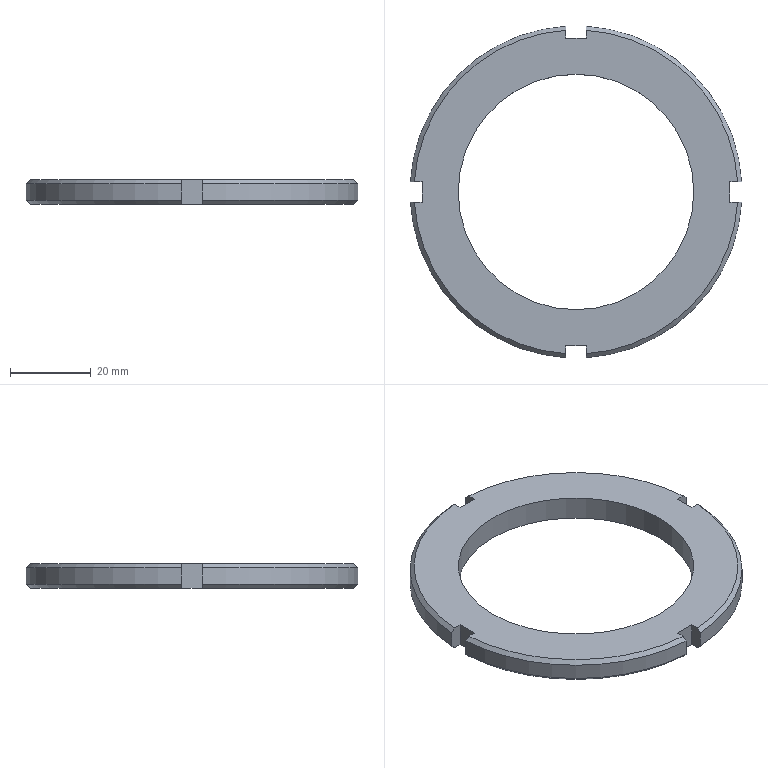Part | NX | features DATUM_CSYS 2, CHAMFER 1, EXTRUDE 1, HOLE PACKAGE 1, Pattern Face Feature 1, SIMPLE HOLE 1, SKETCH 1, SYMBOLIC_THREAD 1 | 1 solid | 27 faces | box 81.847 x 81.847 x 6 mm | volume 15157 mm3 | plane 14 | cone 8 | cylinder 5 | commonest cylinder face diameters 82 x4 58.154 x1
STEP:
#1=CARTESIAN_POINT('',(-2.5,40.924,5.));
#2=VERTEX_POINT('',#1);
#3=CARTESIAN_POINT('',(-2.5,40.924,1.));
#4=VERTEX_POINT('',#3);
#5=CARTESIAN_POINT('',(-2.5,40.924,6.));
#6=DIRECTION('',(0.,0.,-1.));
#7=VECTOR('',#6,1000.);
#8=LINE('',#5,#7);
#9=EDGE_CURVE('',#2,#4,#8,.T.);
#10=ORIENTED_EDGE('',*,*,#9,.T.);
#11=CARTESIAN_POINT('',(-40.924,2.5,1.));
#12=VERTEX_POINT('',#11);
#13=CARTESIAN_POINT('',(0.,0.,1.));
#14=DIRECTION('',(0.,0.,1.));
#15=DIRECTION('',(1.,0.,0.));
#16=AXIS2_PLACEMENT_3D('',#13,#14,#15);
#17=CIRCLE('',#16,41.);
#18=EDGE_CURVE('',#4,#12,#17,.T.);
#19=ORIENTED_EDGE('',*,*,#18,.T.);
#20=CARTESIAN_POINT('',(-40.924,2.5,5.));
#21=VERTEX_POINT('',#20);
#22=CARTESIAN_POINT('',(-40.924,2.5,6.));
#23=DIRECTION('',(0.,0.,-1.));
#24=VECTOR('',#23,1000.);
#25=LINE('',#22,#24);
#26=EDGE_CURVE('',#21,#12,#25,.T.);
#27=ORIENTED_EDGE('',*,*,#26,.F.);
#28=CARTESIAN_POINT('',(0.,0.,5.));
#29=DIRECTION('',(0.,0.,1.));
#30=DIRECTION('',(1.,0.,0.));
#31=AXIS2_PLACEMENT_3D('',#28,#29,#30);
#32=CIRCLE('',#31,41.);
#33=EDGE_CURVE('',#21,#2,#32,.F.);
#34=ORIENTED_EDGE('',*,*,#33,.T.);
#35=EDGE_LOOP('',(#10,#19,#27,#34));
#36=FACE_BOUND('',#35,.T.);
#37=CARTESIAN_POINT('',(0.,0.,6.));
#38=DIRECTION('',(0.,0.,-1.));
#39=DIRECTION('',(-1.,0.,0.));
#40=AXIS2_PLACEMENT_3D('',#37,#38,#39);
#41=CYLINDRICAL_SURFACE('',#40,41.);
#42=ADVANCED_FACE('',(#36),#41,.T.);
#43=CARTESIAN_POINT('',(2.5,40.924,5.));
#44=VERTEX_POINT('',#43);
#45=CARTESIAN_POINT('',(2.5,40.924,1.));
#46=VERTEX_POINT('',#45);
#47=CARTESIAN_POINT('',(2.5,40.924,6.));
#48=DIRECTION('',(0.,0.,-1.));
#49=VECTOR('',#48,1000.);
#50=LINE('',#47,#49);
#51=EDGE_CURVE('',#44,#46,#50,.T.);
#52=ORIENTED_EDGE('',*,*,#51,.T.);
#53=CARTESIAN_POINT('',(2.5,39.922,0.));
#54=VERTEX_POINT('',#53);
#55=CARTESIAN_POINT('',(2.5,40.924,1.));
#56=CARTESIAN_POINT('',(2.5,40.59,0.6667));
#57=CARTESIAN_POINT('',(2.5,40.256,0.3333));
#58=CARTESIAN_POINT('',(2.5,39.922,0.));
#59=B_SPLINE_CURVE_WITH_KNOTS('',3,(#55,#56,#57,#58),.UNSPECIFIED.,.F.,.F.,(4,4),(0.,0.001416),.UNSPECIFIED.);
#60=EDGE_CURVE('',#46,#54,#59,.T.);
#61=ORIENTED_EDGE('',*,*,#60,.T.);
#62=CARTESIAN_POINT('',(2.5,38.,0.));
#63=VERTEX_POINT('',#62);
#64=CARTESIAN_POINT('',(2.5,40.924,0.));
#65=DIRECTION('',(0.,-1.,0.));
#66=VECTOR('',#65,1000.);
#67=LINE('',#64,#66);
#68=EDGE_CURVE('',#54,#63,#67,.T.);
#69=ORIENTED_EDGE('',*,*,#68,.T.);
#70=CARTESIAN_POINT('',(2.5,38.,6.));
#71=VERTEX_POINT('',#70);
#72=CARTESIAN_POINT('',(2.5,38.,6.));
#73=DIRECTION('',(0.,0.,-1.));
#74=VECTOR('',#73,1000.);
#75=LINE('',#72,#74);
#76=EDGE_CURVE('',#71,#63,#75,.T.);
#77=ORIENTED_EDGE('',*,*,#76,.F.);
#78=CARTESIAN_POINT('',(2.5,39.922,6.));
#79=VERTEX_POINT('',#78);
#80=CARTESIAN_POINT('',(2.5,40.924,6.));
#81=DIRECTION('',(0.,-1.,0.));
#82=VECTOR('',#81,1000.);
#83=LINE('',#80,#82);
#84=EDGE_CURVE('',#79,#71,#83,.T.);
#85=ORIENTED_EDGE('',*,*,#84,.F.);
#86=CARTESIAN_POINT('',(2.5,39.922,6.));
#87=CARTESIAN_POINT('',(2.5,40.256,5.667));
#88=CARTESIAN_POINT('',(2.5,40.59,5.333));
#89=CARTESIAN_POINT('',(2.5,40.924,5.));
#90=B_SPLINE_CURVE_WITH_KNOTS('',3,(#86,#87,#88,#89),.UNSPECIFIED.,.F.,.F.,(4,4),(0.,0.001416),.UNSPECIFIED.);
#91=EDGE_CURVE('',#79,#44,#90,.T.);
#92=ORIENTED_EDGE('',*,*,#91,.T.);
#93=EDGE_LOOP('',(#52,#61,#69,#77,#85,#92));
#94=FACE_BOUND('',#93,.T.);
#95=CARTESIAN_POINT('',(2.5,40.924,6.));
#96=DIRECTION('',(1.,0.,0.));
#97=DIRECTION('',(0.,1.,0.));
#98=AXIS2_PLACEMENT_3D('',#95,#96,#97);
#99=PLANE('',#98);
#100=ADVANCED_FACE('',(#94),#99,.F.);
#101=CARTESIAN_POINT('',(-2.5,38.,0.));
#102=VERTEX_POINT('',#101);
#103=CARTESIAN_POINT('',(2.5,38.,0.));
#104=DIRECTION('',(-1.,0.,0.));
#105=VECTOR('',#104,1000.);
#106=LINE('',#103,#105);
#107=EDGE_CURVE('',#63,#102,#106,.T.);
#108=ORIENTED_EDGE('',*,*,#107,.T.);
#109=CARTESIAN_POINT('',(-2.5,38.,6.));
#110=VERTEX_POINT('',#109);
#111=CARTESIAN_POINT('',(-2.5,38.,6.));
#112=DIRECTION('',(0.,0.,-1.));
#113=VECTOR('',#112,1000.);
#114=LINE('',#111,#113);
#115=EDGE_CURVE('',#110,#102,#114,.T.);
#116=ORIENTED_EDGE('',*,*,#115,.F.);
#117=CARTESIAN_POINT('',(2.5,38.,6.));
#118=DIRECTION('',(-1.,0.,0.));
#119=VECTOR('',#118,1000.);
#120=LINE('',#117,#119);
#121=EDGE_CURVE('',#71,#110,#120,.T.);
#122=ORIENTED_EDGE('',*,*,#121,.F.);
#123=ORIENTED_EDGE('',*,*,#76,.T.);
#124=EDGE_LOOP('',(#108,#116,#122,#123));
#125=FACE_BOUND('',#124,.T.);
#126=CARTESIAN_POINT('',(2.5,38.,6.));
#127=DIRECTION('',(0.,-1.,0.));
#128=DIRECTION('',(0.,0.,1.));
#129=AXIS2_PLACEMENT_3D('',#126,#127,#128);
#130=PLANE('',#129);
#131=ADVANCED_FACE('',(#125),#130,.F.);
#132=CARTESIAN_POINT('',(-2.5,39.922,0.));
#133=VERTEX_POINT('',#132);
#134=CARTESIAN_POINT('',(-2.5,38.,0.));
#135=DIRECTION('',(0.,1.,0.));
#136=VECTOR('',#135,1000.);
#137=LINE('',#134,#136);
#138=EDGE_CURVE('',#102,#133,#137,.T.);
#139=ORIENTED_EDGE('',*,*,#138,.T.);
#140=CARTESIAN_POINT('',(-2.5,39.922,0.));
#141=CARTESIAN_POINT('',(-2.5,40.256,0.3333));
#142=CARTESIAN_POINT('',(-2.5,40.59,0.6667));
#143=CARTESIAN_POINT('',(-2.5,40.924,1.));
#144=B_SPLINE_CURVE_WITH_KNOTS('',3,(#140,#141,#142,#143),.UNSPECIFIED.,.F.,.F.,(4,4),(0.,0.001416),.UNSPECIFIED.);
#145=EDGE_CURVE('',#133,#4,#144,.T.);
#146=ORIENTED_EDGE('',*,*,#145,.T.);
#147=ORIENTED_EDGE('',*,*,#9,.F.);
#148=CARTESIAN_POINT('',(-2.5,39.922,6.));
#149=VERTEX_POINT('',#148);
#150=CARTESIAN_POINT('',(-2.5,40.924,5.));
#151=CARTESIAN_POINT('',(-2.5,40.59,5.333));
#152=CARTESIAN_POINT('',(-2.5,40.256,5.667));
#153=CARTESIAN_POINT('',(-2.5,39.922,6.));
#154=B_SPLINE_CURVE_WITH_KNOTS('',3,(#150,#151,#152,#153),.UNSPECIFIED.,.F.,.F.,(4,4),(0.,0.001416),.UNSPECIFIED.);
#155=EDGE_CURVE('',#2,#149,#154,.T.);
#156=ORIENTED_EDGE('',*,*,#155,.T.);
#157=CARTESIAN_POINT('',(-2.5,38.,6.));
#158=DIRECTION('',(0.,1.,0.));
#159=VECTOR('',#158,1000.);
#160=LINE('',#157,#159);
#161=EDGE_CURVE('',#110,#149,#160,.T.);
#162=ORIENTED_EDGE('',*,*,#161,.F.);
#163=ORIENTED_EDGE('',*,*,#115,.T.);
#164=EDGE_LOOP('',(#139,#146,#147,#156,#162,#163));
#165=FACE_BOUND('',#164,.T.);
#166=CARTESIAN_POINT('',(-2.5,38.,6.));
#167=DIRECTION('',(-1.,0.,0.));
#168=DIRECTION('',(0.,-1.,0.));
#169=AXIS2_PLACEMENT_3D('',#166,#167,#168);
#170=PLANE('',#169);
#171=ADVANCED_FACE('',(#165),#170,.F.);
#172=CARTESIAN_POINT('',(-40.924,-2.5,5.));
#173=VERTEX_POINT('',#172);
#174=CARTESIAN_POINT('',(-40.924,-2.5,1.));
#175=VERTEX_POINT('',#174);
#176=CARTESIAN_POINT('',(-40.924,-2.5,6.));
#177=DIRECTION('',(0.,0.,-1.));
#178=VECTOR('',#177,1000.);
#179=LINE('',#176,#178);
#180=EDGE_CURVE('',#173,#175,#179,.T.);
#181=ORIENTED_EDGE('',*,*,#180,.T.);
#182=CARTESIAN_POINT('',(-2.5,-40.924,1.));
#183=VERTEX_POINT('',#182);
#184=CARTESIAN_POINT('',(0.,0.,1.));
#185=DIRECTION('',(0.,0.,1.));
#186=DIRECTION('',(1.,0.,0.));
#187=AXIS2_PLACEMENT_3D('',#184,#185,#186);
#188=CIRCLE('',#187,41.);
#189=EDGE_CURVE('',#175,#183,#188,.T.);
#190=ORIENTED_EDGE('',*,*,#189,.T.);
#191=CARTESIAN_POINT('',(-2.5,-40.924,5.));
#192=VERTEX_POINT('',#191);
#193=CARTESIAN_POINT('',(-2.5,-40.924,6.));
#194=DIRECTION('',(0.,0.,-1.));
#195=VECTOR('',#194,1000.);
#196=LINE('',#193,#195);
#197=EDGE_CURVE('',#192,#183,#196,.T.);
#198=ORIENTED_EDGE('',*,*,#197,.F.);
#199=CARTESIAN_POINT('',(0.,0.,5.));
#200=DIRECTION('',(0.,0.,1.));
#201=DIRECTION('',(1.,0.,0.));
#202=AXIS2_PLACEMENT_3D('',#199,#200,#201);
#203=CIRCLE('',#202,41.);
#204=EDGE_CURVE('',#192,#173,#203,.F.);
#205=ORIENTED_EDGE('',*,*,#204,.T.);
#206=EDGE_LOOP('',(#181,#190,#198,#205));
#207=FACE_BOUND('',#206,.T.);
#208=CARTESIAN_POINT('',(0.,0.,6.));
#209=DIRECTION('',(0.,0.,-1.));
#210=DIRECTION('',(-1.,0.,0.));
#211=AXIS2_PLACEMENT_3D('',#208,#209,#210);
#212=CYLINDRICAL_SURFACE('',#211,41.);
#213=ADVANCED_FACE('',(#207),#212,.T.);
#214=ORIENTED_EDGE('',*,*,#26,.T.);
#215=CARTESIAN_POINT('',(-39.922,2.5,0.));
#216=VERTEX_POINT('',#215);
#217=CARTESIAN_POINT('',(-40.924,2.5,1.));
#218=CARTESIAN_POINT('',(-40.59,2.5,0.6667));
#219=CARTESIAN_POINT('',(-40.256,2.5,0.3333));
#220=CARTESIAN_POINT('',(-39.922,2.5,0.));
#221=B_SPLINE_CURVE_WITH_KNOTS('',3,(#217,#218,#219,#220),.UNSPECIFIED.,.F.,.F.,(4,4),(0.,0.001416),.UNSPECIFIED.);
#222=EDGE_CURVE('',#12,#216,#221,.T.);
#223=ORIENTED_EDGE('',*,*,#222,.T.);
#224=CARTESIAN_POINT('',(-38.,2.5,0.));
#225=VERTEX_POINT('',#224);
#226=CARTESIAN_POINT('',(-40.924,2.5,0.));
#227=DIRECTION('',(1.,0.,0.));
#228=VECTOR('',#227,1000.);
#229=LINE('',#226,#228);
#230=EDGE_CURVE('',#216,#225,#229,.T.);
#231=ORIENTED_EDGE('',*,*,#230,.T.);
#232=CARTESIAN_POINT('',(-38.,2.5,6.));
#233=VERTEX_POINT('',#232);
#234=CARTESIAN_POINT('',(-38.,2.5,6.));
#235=DIRECTION('',(0.,0.,-1.));
#236=VECTOR('',#235,1000.);
#237=LINE('',#234,#236);
#238=EDGE_CURVE('',#233,#225,#237,.T.);
#239=ORIENTED_EDGE('',*,*,#238,.F.);
#240=CARTESIAN_POINT('',(-39.922,2.5,6.));
#241=VERTEX_POINT('',#240);
#242=CARTESIAN_POINT('',(-40.924,2.5,6.));
#243=DIRECTION('',(1.,0.,0.));
#244=VECTOR('',#243,1000.);
#245=LINE('',#242,#244);
#246=EDGE_CURVE('',#241,#233,#245,.T.);
#247=ORIENTED_EDGE('',*,*,#246,.F.);
#248=CARTESIAN_POINT('',(-39.922,2.5,6.));
#249=CARTESIAN_POINT('',(-40.256,2.5,5.667));
#250=CARTESIAN_POINT('',(-40.59,2.5,5.333));
#251=CARTESIAN_POINT('',(-40.924,2.5,5.));
#252=B_SPLINE_CURVE_WITH_KNOTS('',3,(#248,#249,#250,#251),.UNSPECIFIED.,.F.,.F.,(4,4),(0.,0.001416),.UNSPECIFIED.);
#253=EDGE_CURVE('',#241,#21,#252,.T.);
#254=ORIENTED_EDGE('',*,*,#253,.T.);
#255=EDGE_LOOP('',(#214,#223,#231,#239,#247,#254));
#256=FACE_BOUND('',#255,.T.);
#257=CARTESIAN_POINT('',(-40.924,2.5,6.));
#258=DIRECTION('',(0.,1.,0.));
#259=DIRECTION('',(-1.,0.,0.));
#260=AXIS2_PLACEMENT_3D('',#257,#258,#259);
#261=PLANE('',#260);
#262=ADVANCED_FACE('',(#256),#261,.F.);
#263=CARTESIAN_POINT('',(-38.,-2.5,0.));
#264=VERTEX_POINT('',#263);
#265=CARTESIAN_POINT('',(-38.,2.5,0.));
#266=DIRECTION('',(0.,-1.,0.));
#267=VECTOR('',#266,1000.);
#268=LINE('',#265,#267);
#269=EDGE_CURVE('',#225,#264,#268,.T.);
#270=ORIENTED_EDGE('',*,*,#269,.T.);
#271=CARTESIAN_POINT('',(-38.,-2.5,6.));
#272=VERTEX_POINT('',#271);
#273=CARTESIAN_POINT('',(-38.,-2.5,6.));
#274=DIRECTION('',(0.,0.,-1.));
#275=VECTOR('',#274,1000.);
#276=LINE('',#273,#275);
#277=EDGE_CURVE('',#272,#264,#276,.T.);
#278=ORIENTED_EDGE('',*,*,#277,.F.);
#279=CARTESIAN_POINT('',(-38.,2.5,6.));
#280=DIRECTION('',(0.,-1.,0.));
#281=VECTOR('',#280,1000.);
#282=LINE('',#279,#281);
#283=EDGE_CURVE('',#233,#272,#282,.T.);
#284=ORIENTED_EDGE('',*,*,#283,.F.);
#285=ORIENTED_EDGE('',*,*,#238,.T.);
#286=EDGE_LOOP('',(#270,#278,#284,#285));
#287=FACE_BOUND('',#286,.T.);
#288=CARTESIAN_POINT('',(-38.,2.5,6.));
#289=DIRECTION('',(1.,0.,0.));
#290=DIRECTION('',(0.,0.,1.));
#291=AXIS2_PLACEMENT_3D('',#288,#289,#290);
#292=PLANE('',#291);
#293=ADVANCED_FACE('',(#287),#292,.F.);
#294=CARTESIAN_POINT('',(-39.922,-2.5,0.));
#295=VERTEX_POINT('',#294);
#296=CARTESIAN_POINT('',(-38.,-2.5,0.));
#297=DIRECTION('',(-1.,0.,0.));
#298=VECTOR('',#297,1000.);
#299=LINE('',#296,#298);
#300=EDGE_CURVE('',#264,#295,#299,.T.);
#301=ORIENTED_EDGE('',*,*,#300,.T.);
#302=CARTESIAN_POINT('',(-39.922,-2.5,0.));
#303=CARTESIAN_POINT('',(-40.256,-2.5,0.3333));
#304=CARTESIAN_POINT('',(-40.59,-2.5,0.6667));
#305=CARTESIAN_POINT('',(-40.924,-2.5,1.));
#306=B_SPLINE_CURVE_WITH_KNOTS('',3,(#302,#303,#304,#305),.UNSPECIFIED.,.F.,.F.,(4,4),(0.,0.001416),.UNSPECIFIED.);
#307=EDGE_CURVE('',#295,#175,#306,.T.);
#308=ORIENTED_EDGE('',*,*,#307,.T.);
#309=ORIENTED_EDGE('',*,*,#180,.F.);
#310=CARTESIAN_POINT('',(-39.922,-2.5,6.));
#311=VERTEX_POINT('',#310);
#312=CARTESIAN_POINT('',(-40.924,-2.5,5.));
#313=CARTESIAN_POINT('',(-40.59,-2.5,5.333));
#314=CARTESIAN_POINT('',(-40.256,-2.5,5.667));
#315=CARTESIAN_POINT('',(-39.922,-2.5,6.));
#316=B_SPLINE_CURVE_WITH_KNOTS('',3,(#312,#313,#314,#315),.UNSPECIFIED.,.F.,.F.,(4,4),(0.,0.001416),.UNSPECIFIED.);
#317=EDGE_CURVE('',#173,#311,#316,.T.);
#318=ORIENTED_EDGE('',*,*,#317,.T.);
#319=CARTESIAN_POINT('',(-38.,-2.5,6.));
#320=DIRECTION('',(-1.,0.,0.));
#321=VECTOR('',#320,1000.);
#322=LINE('',#319,#321);
#323=EDGE_CURVE('',#272,#311,#322,.T.);
#324=ORIENTED_EDGE('',*,*,#323,.F.);
#325=ORIENTED_EDGE('',*,*,#277,.T.);
#326=EDGE_LOOP('',(#301,#308,#309,#318,#324,#325));
#327=FACE_BOUND('',#326,.T.);
#328=CARTESIAN_POINT('',(-38.,-2.5,6.));
#329=DIRECTION('',(0.,-1.,0.));
#330=DIRECTION('',(1.,0.,0.));
#331=AXIS2_PLACEMENT_3D('',#328,#329,#330);
#332=PLANE('',#331);
#333=ADVANCED_FACE('',(#327),#332,.F.);
#334=CARTESIAN_POINT('',(2.5,-40.924,5.));
#335=VERTEX_POINT('',#334);
#336=CARTESIAN_POINT('',(2.5,-40.924,1.));
#337=VERTEX_POINT('',#336);
#338=CARTESIAN_POINT('',(2.5,-40.924,6.));
#339=DIRECTION('',(0.,0.,-1.));
#340=VECTOR('',#339,1000.);
#341=LINE('',#338,#340);
#342=EDGE_CURVE('',#335,#337,#341,.T.);
#343=ORIENTED_EDGE('',*,*,#342,.T.);
#344=CARTESIAN_POINT('',(40.924,-2.5,1.));
#345=VERTEX_POINT('',#344);
#346=CARTESIAN_POINT('',(0.,0.,1.));
#347=DIRECTION('',(0.,0.,1.));
#348=DIRECTION('',(1.,0.,0.));
#349=AXIS2_PLACEMENT_3D('',#346,#347,#348);
#350=CIRCLE('',#349,41.);
#351=EDGE_CURVE('',#337,#345,#350,.T.);
#352=ORIENTED_EDGE('',*,*,#351,.T.);
#353=CARTESIAN_POINT('',(40.924,-2.5,5.));
#354=VERTEX_POINT('',#353);
#355=CARTESIAN_POINT('',(40.924,-2.5,6.));
#356=DIRECTION('',(0.,0.,-1.));
#357=VECTOR('',#356,1000.);
#358=LINE('',#355,#357);
#359=EDGE_CURVE('',#354,#345,#358,.T.);
#360=ORIENTED_EDGE('',*,*,#359,.F.);
#361=CARTESIAN_POINT('',(0.,0.,5.));
#362=DIRECTION('',(0.,0.,1.));
#363=DIRECTION('',(1.,0.,0.));
#364=AXIS2_PLACEMENT_3D('',#361,#362,#363);
#365=CIRCLE('',#364,41.);
#366=EDGE_CURVE('',#354,#335,#365,.F.);
#367=ORIENTED_EDGE('',*,*,#366,.T.);
#368=EDGE_LOOP('',(#343,#352,#360,#367));
#369=FACE_BOUND('',#368,.T.);
#370=CARTESIAN_POINT('',(0.,0.,6.));
#371=DIRECTION('',(0.,0.,-1.));
#372=DIRECTION('',(-1.,0.,0.));
#373=AXIS2_PLACEMENT_3D('',#370,#371,#372);
#374=CYLINDRICAL_SURFACE('',#373,41.);
#375=ADVANCED_FACE('',(#369),#374,.T.);
#376=ORIENTED_EDGE('',*,*,#197,.T.);
#377=CARTESIAN_POINT('',(-2.5,-39.922,0.));
#378=VERTEX_POINT('',#377);
#379=CARTESIAN_POINT('',(-2.5,-40.924,1.));
#380=CARTESIAN_POINT('',(-2.5,-40.59,0.6667));
#381=CARTESIAN_POINT('',(-2.5,-40.256,0.3333));
#382=CARTESIAN_POINT('',(-2.5,-39.922,0.));
#383=B_SPLINE_CURVE_WITH_KNOTS('',3,(#379,#380,#381,#382),.UNSPECIFIED.,.F.,.F.,(4,4),(0.,0.001416),.UNSPECIFIED.);
#384=EDGE_CURVE('',#183,#378,#383,.T.);
#385=ORIENTED_EDGE('',*,*,#384,.T.);
#386=CARTESIAN_POINT('',(-2.5,-38.,0.));
#387=VERTEX_POINT('',#386);
#388=CARTESIAN_POINT('',(-2.5,-40.924,0.));
#389=DIRECTION('',(0.,1.,0.));
#390=VECTOR('',#389,1000.);
#391=LINE('',#388,#390);
#392=EDGE_CURVE('',#378,#387,#391,.T.);
#393=ORIENTED_EDGE('',*,*,#392,.T.);
#394=CARTESIAN_POINT('',(-2.5,-38.,6.));
#395=VERTEX_POINT('',#394);
#396=CARTESIAN_POINT('',(-2.5,-38.,6.));
#397=DIRECTION('',(0.,0.,-1.));
#398=VECTOR('',#397,1000.);
#399=LINE('',#396,#398);
#400=EDGE_CURVE('',#395,#387,#399,.T.);
#401=ORIENTED_EDGE('',*,*,#400,.F.);
#402=CARTESIAN_POINT('',(-2.5,-39.922,6.));
#403=VERTEX_POINT('',#402);
#404=CARTESIAN_POINT('',(-2.5,-40.924,6.));
#405=DIRECTION('',(0.,1.,0.));
#406=VECTOR('',#405,1000.);
#407=LINE('',#404,#406);
#408=EDGE_CURVE('',#403,#395,#407,.T.);
#409=ORIENTED_EDGE('',*,*,#408,.F.);
#410=CARTESIAN_POINT('',(-2.5,-39.922,6.));
#411=CARTESIAN_POINT('',(-2.5,-40.256,5.667));
#412=CARTESIAN_POINT('',(-2.5,-40.59,5.333));
#413=CARTESIAN_POINT('',(-2.5,-40.924,5.));
#414=B_SPLINE_CURVE_WITH_KNOTS('',3,(#410,#411,#412,#413),.UNSPECIFIED.,.F.,.F.,(4,4),(0.,0.001416),.UNSPECIFIED.);
#415=EDGE_CURVE('',#403,#192,#414,.T.);
#416=ORIENTED_EDGE('',*,*,#415,.T.);
#417=EDGE_LOOP('',(#376,#385,#393,#401,#409,#416));
#418=FACE_BOUND('',#417,.T.);
#419=CARTESIAN_POINT('',(-2.5,-40.924,6.));
#420=DIRECTION('',(-1.,0.,0.));
#421=DIRECTION('',(0.,-1.,0.));
#422=AXIS2_PLACEMENT_3D('',#419,#420,#421);
#423=PLANE('',#422);
#424=ADVANCED_FACE('',(#418),#423,.F.);
#425=CARTESIAN_POINT('',(2.5,-38.,0.));
#426=VERTEX_POINT('',#425);
#427=CARTESIAN_POINT('',(-2.5,-38.,0.));
#428=DIRECTION('',(1.,0.,0.));
#429=VECTOR('',#428,1000.);
#430=LINE('',#427,#429);
#431=EDGE_CURVE('',#387,#426,#430,.T.);
#432=ORIENTED_EDGE('',*,*,#431,.T.);
#433=CARTESIAN_POINT('',(2.5,-38.,6.));
#434=VERTEX_POINT('',#433);
#435=CARTESIAN_POINT('',(2.5,-38.,6.));
#436=DIRECTION('',(0.,0.,-1.));
#437=VECTOR('',#436,1000.);
#438=LINE('',#435,#437);
#439=EDGE_CURVE('',#434,#426,#438,.T.);
#440=ORIENTED_EDGE('',*,*,#439,.F.);
#441=CARTESIAN_POINT('',(-2.5,-38.,6.));
#442=DIRECTION('',(1.,0.,0.));
#443=VECTOR('',#442,1000.);
#444=LINE('',#441,#443);
#445=EDGE_CURVE('',#395,#434,#444,.T.);
#446=ORIENTED_EDGE('',*,*,#445,.F.);
#447=ORIENTED_EDGE('',*,*,#400,.T.);
#448=EDGE_LOOP('',(#432,#440,#446,#447));
#449=FACE_BOUND('',#448,.T.);
#450=CARTESIAN_POINT('',(-2.5,-38.,6.));
#451=DIRECTION('',(0.,1.,0.));
#452=DIRECTION('',(0.,0.,1.));
#453=AXIS2_PLACEMENT_3D('',#450,#451,#452);
#454=PLANE('',#453);
#455=ADVANCED_FACE('',(#449),#454,.F.);
#456=CARTESIAN_POINT('',(2.5,-39.922,0.));
#457=VERTEX_POINT('',#456);
#458=CARTESIAN_POINT('',(2.5,-38.,0.));
#459=DIRECTION('',(0.,-1.,0.));
#460=VECTOR('',#459,1000.);
#461=LINE('',#458,#460);
#462=EDGE_CURVE('',#426,#457,#461,.T.);
#463=ORIENTED_EDGE('',*,*,#462,.T.);
#464=CARTESIAN_POINT('',(2.5,-39.922,0.));
#465=CARTESIAN_POINT('',(2.5,-40.256,0.3333));
#466=CARTESIAN_POINT('',(2.5,-40.59,0.6667));
#467=CARTESIAN_POINT('',(2.5,-40.924,1.));
#468=B_SPLINE_CURVE_WITH_KNOTS('',3,(#464,#465,#466,#467),.UNSPECIFIED.,.F.,.F.,(4,4),(0.,0.001416),.UNSPECIFIED.);
#469=EDGE_CURVE('',#457,#337,#468,.T.);
#470=ORIENTED_EDGE('',*,*,#469,.T.);
#471=ORIENTED_EDGE('',*,*,#342,.F.);
#472=CARTESIAN_POINT('',(2.5,-39.922,6.));
#473=VERTEX_POINT('',#472);
#474=CARTESIAN_POINT('',(2.5,-40.924,5.));
#475=CARTESIAN_POINT('',(2.5,-40.59,5.333));
#476=CARTESIAN_POINT('',(2.5,-40.256,5.667));
#477=CARTESIAN_POINT('',(2.5,-39.922,6.));
#478=B_SPLINE_CURVE_WITH_KNOTS('',3,(#474,#475,#476,#477),.UNSPECIFIED.,.F.,.F.,(4,4),(0.,0.001416),.UNSPECIFIED.);
#479=EDGE_CURVE('',#335,#473,#478,.T.);
#480=ORIENTED_EDGE('',*,*,#479,.T.);
#481=CARTESIAN_POINT('',(2.5,-38.,6.));
#482=DIRECTION('',(0.,-1.,0.));
#483=VECTOR('',#482,1000.);
#484=LINE('',#481,#483);
#485=EDGE_CURVE('',#434,#473,#484,.T.);
#486=ORIENTED_EDGE('',*,*,#485,.F.);
#487=ORIENTED_EDGE('',*,*,#439,.T.);
#488=EDGE_LOOP('',(#463,#470,#471,#480,#486,#487));
#489=FACE_BOUND('',#488,.T.);
#490=CARTESIAN_POINT('',(2.5,-38.,6.));
#491=DIRECTION('',(1.,0.,0.));
#492=DIRECTION('',(0.,1.,0.));
#493=AXIS2_PLACEMENT_3D('',#490,#491,#492);
#494=PLANE('',#493);
#495=ADVANCED_FACE('',(#489),#494,.F.);
#496=CARTESIAN_POINT('',(38.,-2.5,0.));
#497=VERTEX_POINT('',#496);
#498=CARTESIAN_POINT('',(38.,2.5,0.));
#499=VERTEX_POINT('',#498);
#500=CARTESIAN_POINT('',(38.,-2.5,0.));
#501=DIRECTION('',(0.,1.,0.));
#502=VECTOR('',#501,1000.);
#503=LINE('',#500,#502);
#504=EDGE_CURVE('',#497,#499,#503,.T.);
#505=ORIENTED_EDGE('',*,*,#504,.T.);
#506=CARTESIAN_POINT('',(38.,2.5,6.));
#507=VERTEX_POINT('',#506);
#508=CARTESIAN_POINT('',(38.,2.5,6.));
#509=DIRECTION('',(0.,0.,-1.));
#510=VECTOR('',#509,1000.);
#511=LINE('',#508,#510);
#512=EDGE_CURVE('',#507,#499,#511,.T.);
#513=ORIENTED_EDGE('',*,*,#512,.F.);
#514=CARTESIAN_POINT('',(38.,-2.5,6.));
#515=VERTEX_POINT('',#514);
#516=CARTESIAN_POINT('',(38.,-2.5,6.));
#517=DIRECTION('',(0.,1.,0.));
#518=VECTOR('',#517,1000.);
#519=LINE('',#516,#518);
#520=EDGE_CURVE('',#515,#507,#519,.T.);
#521=ORIENTED_EDGE('',*,*,#520,.F.);
#522=CARTESIAN_POINT('',(38.,-2.5,6.));
#523=DIRECTION('',(0.,0.,-1.));
#524=VECTOR('',#523,1000.);
#525=LINE('',#522,#524);
#526=EDGE_CURVE('',#515,#497,#525,.T.);
#527=ORIENTED_EDGE('',*,*,#526,.T.);
#528=EDGE_LOOP('',(#505,#513,#521,#527));
#529=FACE_BOUND('',#528,.T.);
#530=CARTESIAN_POINT('',(38.,-2.5,6.));
#531=DIRECTION('',(-1.,0.,0.));
#532=DIRECTION('',(0.,0.,1.));
#533=AXIS2_PLACEMENT_3D('',#530,#531,#532);
#534=PLANE('',#533);
#535=ADVANCED_FACE('',(#529),#534,.F.);
#536=CARTESIAN_POINT('',(39.922,2.5,0.));
#537=VERTEX_POINT('',#536);
#538=CARTESIAN_POINT('',(38.,2.5,0.));
#539=DIRECTION('',(1.,0.,0.));
#540=VECTOR('',#539,1000.);
#541=LINE('',#538,#540);
#542=EDGE_CURVE('',#499,#537,#541,.T.);
#543=ORIENTED_EDGE('',*,*,#542,.T.);
#544=CARTESIAN_POINT('',(40.924,2.5,1.));
#545=VERTEX_POINT('',#544);
#546=CARTESIAN_POINT('',(39.922,2.5,0.));
#547=CARTESIAN_POINT('',(40.256,2.5,0.3333));
#548=CARTESIAN_POINT('',(40.59,2.5,0.6667));
#549=CARTESIAN_POINT('',(40.924,2.5,1.));
#550=B_SPLINE_CURVE_WITH_KNOTS('',3,(#546,#547,#548,#549),.UNSPECIFIED.,.F.,.F.,(4,4),(0.,0.001416),.UNSPECIFIED.);
#551=EDGE_CURVE('',#537,#545,#550,.T.);
#552=ORIENTED_EDGE('',*,*,#551,.T.);
#553=CARTESIAN_POINT('',(40.924,2.5,5.));
#554=VERTEX_POINT('',#553);
#555=CARTESIAN_POINT('',(40.924,2.5,6.));
#556=DIRECTION('',(0.,0.,-1.));
#557=VECTOR('',#556,1000.);
#558=LINE('',#555,#557);
#559=EDGE_CURVE('',#554,#545,#558,.T.);
#560=ORIENTED_EDGE('',*,*,#559,.F.);
#561=CARTESIAN_POINT('',(39.922,2.5,6.));
#562=VERTEX_POINT('',#561);
#563=CARTESIAN_POINT('',(40.924,2.5,5.));
#564=CARTESIAN_POINT('',(40.59,2.5,5.333));
#565=CARTESIAN_POINT('',(40.256,2.5,5.667));
#566=CARTESIAN_POINT('',(39.922,2.5,6.));
#567=B_SPLINE_CURVE_WITH_KNOTS('',3,(#563,#564,#565,#566),.UNSPECIFIED.,.F.,.F.,(4,4),(0.,0.001416),.UNSPECIFIED.);
#568=EDGE_CURVE('',#554,#562,#567,.T.);
#569=ORIENTED_EDGE('',*,*,#568,.T.);
#570=CARTESIAN_POINT('',(38.,2.5,6.));
#571=DIRECTION('',(1.,0.,0.));
#572=VECTOR('',#571,1000.);
#573=LINE('',#570,#572);
#574=EDGE_CURVE('',#507,#562,#573,.T.);
#575=ORIENTED_EDGE('',*,*,#574,.F.);
#576=ORIENTED_EDGE('',*,*,#512,.T.);
#577=EDGE_LOOP('',(#543,#552,#560,#569,#575,#576));
#578=FACE_BOUND('',#577,.T.);
#579=CARTESIAN_POINT('',(38.,2.5,6.));
#580=DIRECTION('',(0.,1.,0.));
#581=DIRECTION('',(-1.,0.,0.));
#582=AXIS2_PLACEMENT_3D('',#579,#580,#581);
#583=PLANE('',#582);
#584=ADVANCED_FACE('',(#578),#583,.F.);
#585=ORIENTED_EDGE('',*,*,#559,.T.);
#586=CARTESIAN_POINT('',(0.,0.,1.));
#587=DIRECTION('',(0.,0.,1.));
#588=DIRECTION('',(1.,0.,0.));
#589=AXIS2_PLACEMENT_3D('',#586,#587,#588);
#590=CIRCLE('',#589,41.);
#591=EDGE_CURVE('',#545,#46,#590,.T.);
#592=ORIENTED_EDGE('',*,*,#591,.T.);
#593=ORIENTED_EDGE('',*,*,#51,.F.);
#594=CARTESIAN_POINT('',(0.,0.,5.));
#595=DIRECTION('',(0.,0.,1.));
#596=DIRECTION('',(1.,0.,0.));
#597=AXIS2_PLACEMENT_3D('',#594,#595,#596);
#598=CIRCLE('',#597,41.);
#599=EDGE_CURVE('',#44,#554,#598,.F.);
#600=ORIENTED_EDGE('',*,*,#599,.T.);
#601=EDGE_LOOP('',(#585,#592,#593,#600));
#602=FACE_BOUND('',#601,.T.);
#603=CARTESIAN_POINT('',(0.,0.,6.));
#604=DIRECTION('',(0.,0.,-1.));
#605=DIRECTION('',(-1.,0.,0.));
#606=AXIS2_PLACEMENT_3D('',#603,#604,#605);
#607=CYLINDRICAL_SURFACE('',#606,41.);
#608=ADVANCED_FACE('',(#602),#607,.T.);
#609=ORIENTED_EDGE('',*,*,#359,.T.);
#610=CARTESIAN_POINT('',(39.922,-2.5,0.));
#611=VERTEX_POINT('',#610);
#612=CARTESIAN_POINT('',(40.924,-2.5,1.));
#613=CARTESIAN_POINT('',(40.59,-2.5,0.6667));
#614=CARTESIAN_POINT('',(40.256,-2.5,0.3333));
#615=CARTESIAN_POINT('',(39.922,-2.5,0.));
#616=B_SPLINE_CURVE_WITH_KNOTS('',3,(#612,#613,#614,#615),.UNSPECIFIED.,.F.,.F.,(4,4),(0.,0.001416),.UNSPECIFIED.);
#617=EDGE_CURVE('',#345,#611,#616,.T.);
#618=ORIENTED_EDGE('',*,*,#617,.T.);
#619=CARTESIAN_POINT('',(40.924,-2.5,0.));
#620=DIRECTION('',(-1.,0.,0.));
#621=VECTOR('',#620,1000.);
#622=LINE('',#619,#621);
#623=EDGE_CURVE('',#611,#497,#622,.T.);
#624=ORIENTED_EDGE('',*,*,#623,.T.);
#625=ORIENTED_EDGE('',*,*,#526,.F.);
#626=CARTESIAN_POINT('',(39.922,-2.5,6.));
#627=VERTEX_POINT('',#626);
#628=CARTESIAN_POINT('',(40.924,-2.5,6.));
#629=DIRECTION('',(-1.,0.,0.));
#630=VECTOR('',#629,1000.);
#631=LINE('',#628,#630);
#632=EDGE_CURVE('',#627,#515,#631,.T.);
#633=ORIENTED_EDGE('',*,*,#632,.F.);
#634=CARTESIAN_POINT('',(39.922,-2.5,6.));
#635=CARTESIAN_POINT('',(40.256,-2.5,5.667));
#636=CARTESIAN_POINT('',(40.59,-2.5,5.333));
#637=CARTESIAN_POINT('',(40.924,-2.5,5.));
#638=B_SPLINE_CURVE_WITH_KNOTS('',3,(#634,#635,#636,#637),.UNSPECIFIED.,.F.,.F.,(4,4),(0.,0.001416),.UNSPECIFIED.);
#639=EDGE_CURVE('',#627,#354,#638,.T.);
#640=ORIENTED_EDGE('',*,*,#639,.T.);
#641=EDGE_LOOP('',(#609,#618,#624,#625,#633,#640));
#642=FACE_BOUND('',#641,.T.);
#643=CARTESIAN_POINT('',(40.924,-2.5,6.));
#644=DIRECTION('',(0.,-1.,0.));
#645=DIRECTION('',(1.,0.,0.));
#646=AXIS2_PLACEMENT_3D('',#643,#644,#645);
#647=PLANE('',#646);
#648=ADVANCED_FACE('',(#642),#647,.F.);
#649=CARTESIAN_POINT('',(-29.077,0.,6.));
#650=VERTEX_POINT('',#649);
#651=CARTESIAN_POINT('',(0.,0.,6.));
#652=DIRECTION('',(0.,0.,-1.));
#653=DIRECTION('',(-1.,0.,0.));
#654=AXIS2_PLACEMENT_3D('',#651,#652,#653);
#655=CIRCLE('',#654,29.077);
#656=EDGE_CURVE('',#650,#650,#655,.T.);
#657=ORIENTED_EDGE('',*,*,#656,.T.);
#658=EDGE_LOOP('',(#657));
#659=FACE_BOUND('',#658,.T.);
#660=ORIENTED_EDGE('',*,*,#323,.T.);
#661=CARTESIAN_POINT('',(0.,0.,6.));
#662=DIRECTION('',(0.,0.,1.));
#663=DIRECTION('',(1.,0.,0.));
#664=AXIS2_PLACEMENT_3D('',#661,#662,#663);
#665=CIRCLE('',#664,40.);
#666=EDGE_CURVE('',#311,#403,#665,.T.);
#667=ORIENTED_EDGE('',*,*,#666,.T.);
#668=ORIENTED_EDGE('',*,*,#408,.T.);
#669=ORIENTED_EDGE('',*,*,#445,.T.);
#670=ORIENTED_EDGE('',*,*,#485,.T.);
#671=CARTESIAN_POINT('',(0.,0.,6.));
#672=DIRECTION('',(0.,0.,1.));
#673=DIRECTION('',(1.,0.,0.));
#674=AXIS2_PLACEMENT_3D('',#671,#672,#673);
#675=CIRCLE('',#674,40.);
#676=EDGE_CURVE('',#473,#627,#675,.T.);
#677=ORIENTED_EDGE('',*,*,#676,.T.);
#678=ORIENTED_EDGE('',*,*,#632,.T.);
#679=ORIENTED_EDGE('',*,*,#520,.T.);
#680=ORIENTED_EDGE('',*,*,#574,.T.);
#681=CARTESIAN_POINT('',(0.,0.,6.));
#682=DIRECTION('',(0.,0.,1.));
#683=DIRECTION('',(1.,0.,0.));
#684=AXIS2_PLACEMENT_3D('',#681,#682,#683);
#685=CIRCLE('',#684,40.);
#686=EDGE_CURVE('',#562,#79,#685,.T.);
#687=ORIENTED_EDGE('',*,*,#686,.T.);
#688=ORIENTED_EDGE('',*,*,#84,.T.);
#689=ORIENTED_EDGE('',*,*,#121,.T.);
#690=ORIENTED_EDGE('',*,*,#161,.T.);
#691=CARTESIAN_POINT('',(0.,0.,6.));
#692=DIRECTION('',(0.,0.,1.));
#693=DIRECTION('',(1.,0.,0.));
#694=AXIS2_PLACEMENT_3D('',#691,#692,#693);
#695=CIRCLE('',#694,40.);
#696=EDGE_CURVE('',#149,#241,#695,.T.);
#697=ORIENTED_EDGE('',*,*,#696,.T.);
#698=ORIENTED_EDGE('',*,*,#246,.T.);
#699=ORIENTED_EDGE('',*,*,#283,.T.);
#700=EDGE_LOOP('',(#660,#667,#668,#669,#670,#677,#678,#679,#680,#687,#688,#689,#690,#697,#698,#699));
#701=FACE_BOUND('',#700,.T.);
#702=CARTESIAN_POINT('',(0.,0.,6.));
#703=DIRECTION('',(0.,0.,1.));
#704=DIRECTION('',(1.,0.,0.));
#705=AXIS2_PLACEMENT_3D('',#702,#703,#704);
#706=PLANE('',#705);
#707=ADVANCED_FACE('',(#659,#701),#706,.T.);
#708=CARTESIAN_POINT('',(29.077,0.,0.));
#709=VERTEX_POINT('',#708);
#710=CARTESIAN_POINT('',(0.,0.,0.));
#711=DIRECTION('',(0.,0.,1.));
#712=DIRECTION('',(1.,0.,0.));
#713=AXIS2_PLACEMENT_3D('',#710,#711,#712);
#714=CIRCLE('',#713,29.077);
#715=EDGE_CURVE('',#709,#709,#714,.T.);
#716=ORIENTED_EDGE('',*,*,#715,.T.);
#717=EDGE_LOOP('',(#716));
#718=FACE_BOUND('',#717,.T.);
#719=ORIENTED_EDGE('',*,*,#392,.F.);
#720=CARTESIAN_POINT('',(0.,0.,0.));
#721=DIRECTION('',(0.,0.,1.));
#722=DIRECTION('',(1.,0.,0.));
#723=AXIS2_PLACEMENT_3D('',#720,#721,#722);
#724=CIRCLE('',#723,40.);
#725=EDGE_CURVE('',#378,#295,#724,.F.);
#726=ORIENTED_EDGE('',*,*,#725,.T.);
#727=ORIENTED_EDGE('',*,*,#300,.F.);
#728=ORIENTED_EDGE('',*,*,#269,.F.);
#729=ORIENTED_EDGE('',*,*,#230,.F.);
#730=CARTESIAN_POINT('',(0.,0.,0.));
#731=DIRECTION('',(0.,0.,1.));
#732=DIRECTION('',(1.,0.,0.));
#733=AXIS2_PLACEMENT_3D('',#730,#731,#732);
#734=CIRCLE('',#733,40.);
#735=EDGE_CURVE('',#216,#133,#734,.F.);
#736=ORIENTED_EDGE('',*,*,#735,.T.);
#737=ORIENTED_EDGE('',*,*,#138,.F.);
#738=ORIENTED_EDGE('',*,*,#107,.F.);
#739=ORIENTED_EDGE('',*,*,#68,.F.);
#740=CARTESIAN_POINT('',(0.,0.,0.));
#741=DIRECTION('',(0.,0.,1.));
#742=DIRECTION('',(1.,0.,0.));
#743=AXIS2_PLACEMENT_3D('',#740,#741,#742);
#744=CIRCLE('',#743,40.);
#745=EDGE_CURVE('',#54,#537,#744,.F.);
#746=ORIENTED_EDGE('',*,*,#745,.T.);
#747=ORIENTED_EDGE('',*,*,#542,.F.);
#748=ORIENTED_EDGE('',*,*,#504,.F.);
#749=ORIENTED_EDGE('',*,*,#623,.F.);
#750=CARTESIAN_POINT('',(0.,0.,0.));
#751=DIRECTION('',(0.,0.,1.));
#752=DIRECTION('',(1.,0.,0.));
#753=AXIS2_PLACEMENT_3D('',#750,#751,#752);
#754=CIRCLE('',#753,40.);
#755=EDGE_CURVE('',#611,#457,#754,.F.);
#756=ORIENTED_EDGE('',*,*,#755,.T.);
#757=ORIENTED_EDGE('',*,*,#462,.F.);
#758=ORIENTED_EDGE('',*,*,#431,.F.);
#759=EDGE_LOOP('',(#719,#726,#727,#728,#729,#736,#737,#738,#739,#746,#747,#748,#749,#756,#757,#758));
#760=FACE_BOUND('',#759,.T.);
#761=CARTESIAN_POINT('',(0.,0.,0.));
#762=DIRECTION('',(0.,0.,1.));
#763=DIRECTION('',(1.,0.,0.));
#764=AXIS2_PLACEMENT_3D('',#761,#762,#763);
#765=PLANE('',#764);
#766=ADVANCED_FACE('',(#718,#760),#765,.F.);
#767=ORIENTED_EDGE('',*,*,#307,.F.);
#768=ORIENTED_EDGE('',*,*,#725,.F.);
#769=ORIENTED_EDGE('',*,*,#384,.F.);
#770=ORIENTED_EDGE('',*,*,#189,.F.);
#771=EDGE_LOOP('',(#767,#768,#769,#770));
#772=FACE_BOUND('',#771,.T.);
#773=CARTESIAN_POINT('',(0.,0.,1.));
#774=DIRECTION('',(0.,0.,1.));
#775=DIRECTION('',(1.,0.,0.));
#776=AXIS2_PLACEMENT_3D('',#773,#774,#775);
#777=CONICAL_SURFACE('',#776,41.,0.7854);
#778=ADVANCED_FACE('',(#772),#777,.T.);
#779=ORIENTED_EDGE('',*,*,#317,.F.);
#780=ORIENTED_EDGE('',*,*,#204,.F.);
#781=ORIENTED_EDGE('',*,*,#415,.F.);
#782=ORIENTED_EDGE('',*,*,#666,.F.);
#783=EDGE_LOOP('',(#779,#780,#781,#782));
#784=FACE_BOUND('',#783,.T.);
#785=CARTESIAN_POINT('',(0.,0.,6.));
#786=DIRECTION('',(0.,0.,-1.));
#787=DIRECTION('',(-1.,0.,0.));
#788=AXIS2_PLACEMENT_3D('',#785,#786,#787);
#789=CONICAL_SURFACE('',#788,40.,0.7854);
#790=ADVANCED_FACE('',(#784),#789,.T.);
#791=ORIENTED_EDGE('',*,*,#469,.F.);
#792=ORIENTED_EDGE('',*,*,#755,.F.);
#793=ORIENTED_EDGE('',*,*,#617,.F.);
#794=ORIENTED_EDGE('',*,*,#351,.F.);
#795=EDGE_LOOP('',(#791,#792,#793,#794));
#796=FACE_BOUND('',#795,.T.);
#797=CARTESIAN_POINT('',(0.,0.,1.));
#798=DIRECTION('',(0.,0.,1.));
#799=DIRECTION('',(1.,0.,0.));
#800=AXIS2_PLACEMENT_3D('',#797,#798,#799);
#801=CONICAL_SURFACE('',#800,41.,0.7854);
#802=ADVANCED_FACE('',(#796),#801,.T.);
#803=ORIENTED_EDGE('',*,*,#479,.F.);
#804=ORIENTED_EDGE('',*,*,#366,.F.);
#805=ORIENTED_EDGE('',*,*,#639,.F.);
#806=ORIENTED_EDGE('',*,*,#676,.F.);
#807=EDGE_LOOP('',(#803,#804,#805,#806));
#808=FACE_BOUND('',#807,.T.);
#809=CARTESIAN_POINT('',(0.,0.,6.));
#810=DIRECTION('',(0.,0.,-1.));
#811=DIRECTION('',(-1.,0.,0.));
#812=AXIS2_PLACEMENT_3D('',#809,#810,#811);
#813=CONICAL_SURFACE('',#812,40.,0.7854);
#814=ADVANCED_FACE('',(#808),#813,.T.);
#815=ORIENTED_EDGE('',*,*,#145,.F.);
#816=ORIENTED_EDGE('',*,*,#735,.F.);
#817=ORIENTED_EDGE('',*,*,#222,.F.);
#818=ORIENTED_EDGE('',*,*,#18,.F.);
#819=EDGE_LOOP('',(#815,#816,#817,#818));
#820=FACE_BOUND('',#819,.T.);
#821=CARTESIAN_POINT('',(0.,0.,1.));
#822=DIRECTION('',(0.,0.,1.));
#823=DIRECTION('',(1.,0.,0.));
#824=AXIS2_PLACEMENT_3D('',#821,#822,#823);
#825=CONICAL_SURFACE('',#824,41.,0.7854);
#826=ADVANCED_FACE('',(#820),#825,.T.);
#827=ORIENTED_EDGE('',*,*,#155,.F.);
#828=ORIENTED_EDGE('',*,*,#33,.F.);
#829=ORIENTED_EDGE('',*,*,#253,.F.);
#830=ORIENTED_EDGE('',*,*,#696,.F.);
#831=EDGE_LOOP('',(#827,#828,#829,#830));
#832=FACE_BOUND('',#831,.T.);
#833=CARTESIAN_POINT('',(0.,0.,6.));
#834=DIRECTION('',(0.,0.,-1.));
#835=DIRECTION('',(-1.,0.,0.));
#836=AXIS2_PLACEMENT_3D('',#833,#834,#835);
#837=CONICAL_SURFACE('',#836,40.,0.7854);
#838=ADVANCED_FACE('',(#832),#837,.T.);
#839=ORIENTED_EDGE('',*,*,#551,.F.);
#840=ORIENTED_EDGE('',*,*,#745,.F.);
#841=ORIENTED_EDGE('',*,*,#60,.F.);
#842=ORIENTED_EDGE('',*,*,#591,.F.);
#843=EDGE_LOOP('',(#839,#840,#841,#842));
#844=FACE_BOUND('',#843,.T.);
#845=CARTESIAN_POINT('',(0.,0.,1.));
#846=DIRECTION('',(0.,0.,1.));
#847=DIRECTION('',(1.,0.,0.));
#848=AXIS2_PLACEMENT_3D('',#845,#846,#847);
#849=CONICAL_SURFACE('',#848,41.,0.7854);
#850=ADVANCED_FACE('',(#844),#849,.T.);
#851=ORIENTED_EDGE('',*,*,#568,.F.);
#852=ORIENTED_EDGE('',*,*,#599,.F.);
#853=ORIENTED_EDGE('',*,*,#91,.F.);
#854=ORIENTED_EDGE('',*,*,#686,.F.);
#855=EDGE_LOOP('',(#851,#852,#853,#854));
#856=FACE_BOUND('',#855,.T.);
#857=CARTESIAN_POINT('',(0.,0.,6.));
#858=DIRECTION('',(0.,0.,-1.));
#859=DIRECTION('',(-1.,0.,0.));
#860=AXIS2_PLACEMENT_3D('',#857,#858,#859);
#861=CONICAL_SURFACE('',#860,40.,0.7854);
#862=ADVANCED_FACE('',(#856),#861,.T.);
#863=ORIENTED_EDGE('',*,*,#656,.F.);
#864=EDGE_LOOP('',(#863));
#865=FACE_BOUND('',#864,.T.);
#866=ORIENTED_EDGE('',*,*,#715,.F.);
#867=EDGE_LOOP('',(#866));
#868=FACE_BOUND('',#867,.T.);
#869=CARTESIAN_POINT('',(0.,0.,6.));
#870=DIRECTION('',(0.,0.,-1.));
#871=DIRECTION('',(-1.,0.,0.));
#872=AXIS2_PLACEMENT_3D('',#869,#870,#871);
#873=CYLINDRICAL_SURFACE('',#872,29.077);
#874=ADVANCED_FACE('',(#865,#868),#873,.F.);
#875=CLOSED_SHELL('',(#42,#100,#131,#171,#213,#262,#293,#333,#375,#424,#455,#495,#535,#584,#608,#648,#707,#766,#778,#790,#802,#814,#826,#838,#850,#862,#874));
#876=MANIFOLD_SOLID_BREP('',#875);
#877=(LENGTH_UNIT()NAMED_UNIT(*)SI_UNIT(.MILLI.,.METRE.));
#878=UNCERTAINTY_MEASURE_WITH_UNIT(LENGTH_MEASURE(0.0508),#877,'','');
#879=(NAMED_UNIT(*)PLANE_ANGLE_UNIT()SI_UNIT($,.RADIAN.));
#880=(NAMED_UNIT(*)SI_UNIT($,.STERADIAN.)SOLID_ANGLE_UNIT());
#881=(GEOMETRIC_REPRESENTATION_CONTEXT(3)GLOBAL_UNCERTAINTY_ASSIGNED_CONTEXT((#878))GLOBAL_UNIT_ASSIGNED_CONTEXT((#877,#879,#880))REPRESENTATION_CONTEXT('',''));
#882=ADVANCED_BREP_SHAPE_REPRESENTATION('',(#876),#881);